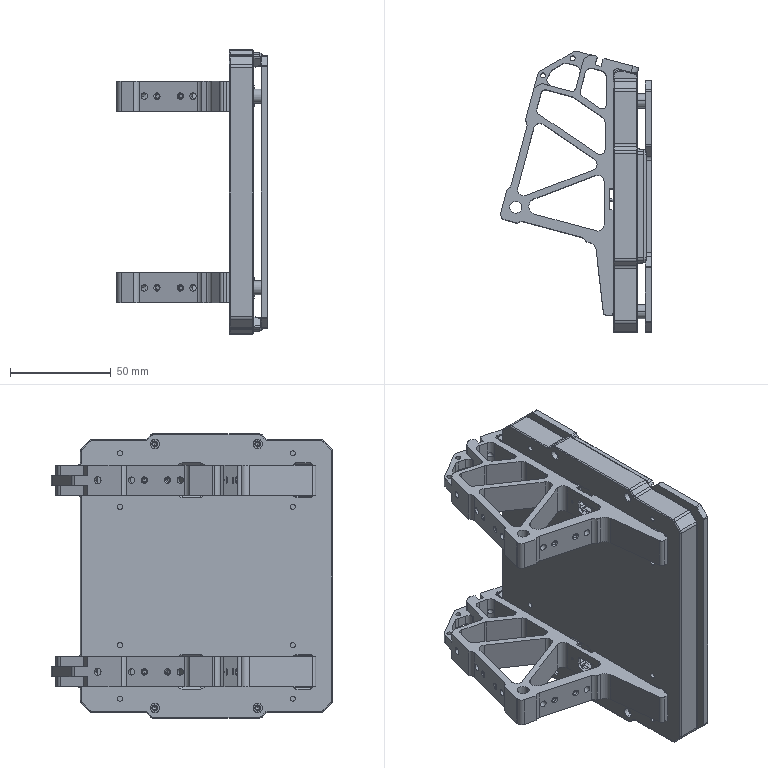Part | SolidWorks | 18 solids | 1655 faces | box 74.786 x 139.379 x 141 mm | volume 156127 mm3 | cylinder 788 | plane 635 | cone 128 | spline 88 | torus 16 | commonest cylinder face diameters 4 x210 1 x119 2 x90 6 x82 3 x36 2.5 x32